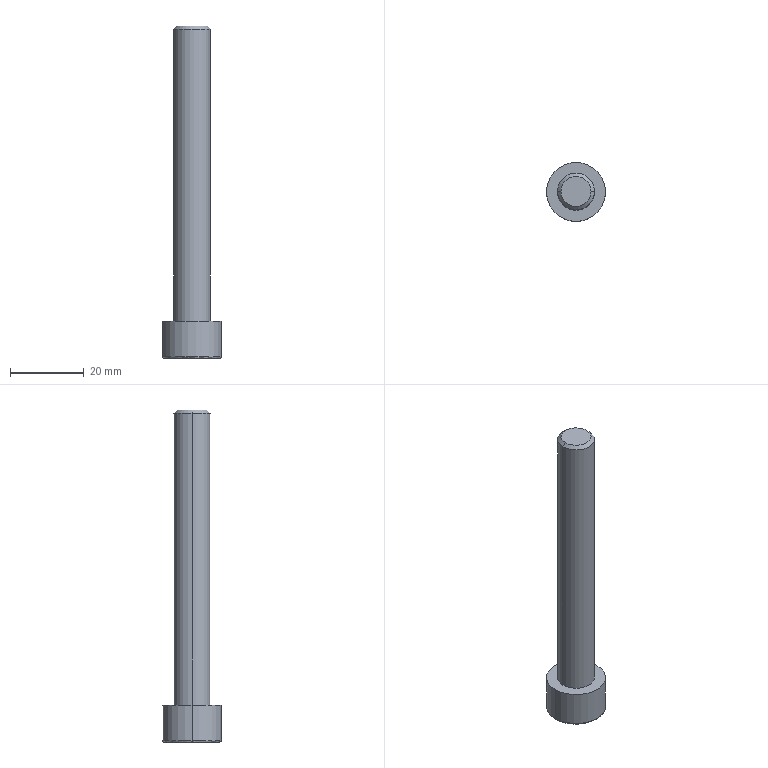Part | STEP file | 23 | 1 solid | 19 faces | box 16 x 16 x 90 mm | volume 7916 mm3 | plane 9 | cylinder 4 | cone 4 | spline 2 | commonest cylinder face diameters 10 x2 16 x2